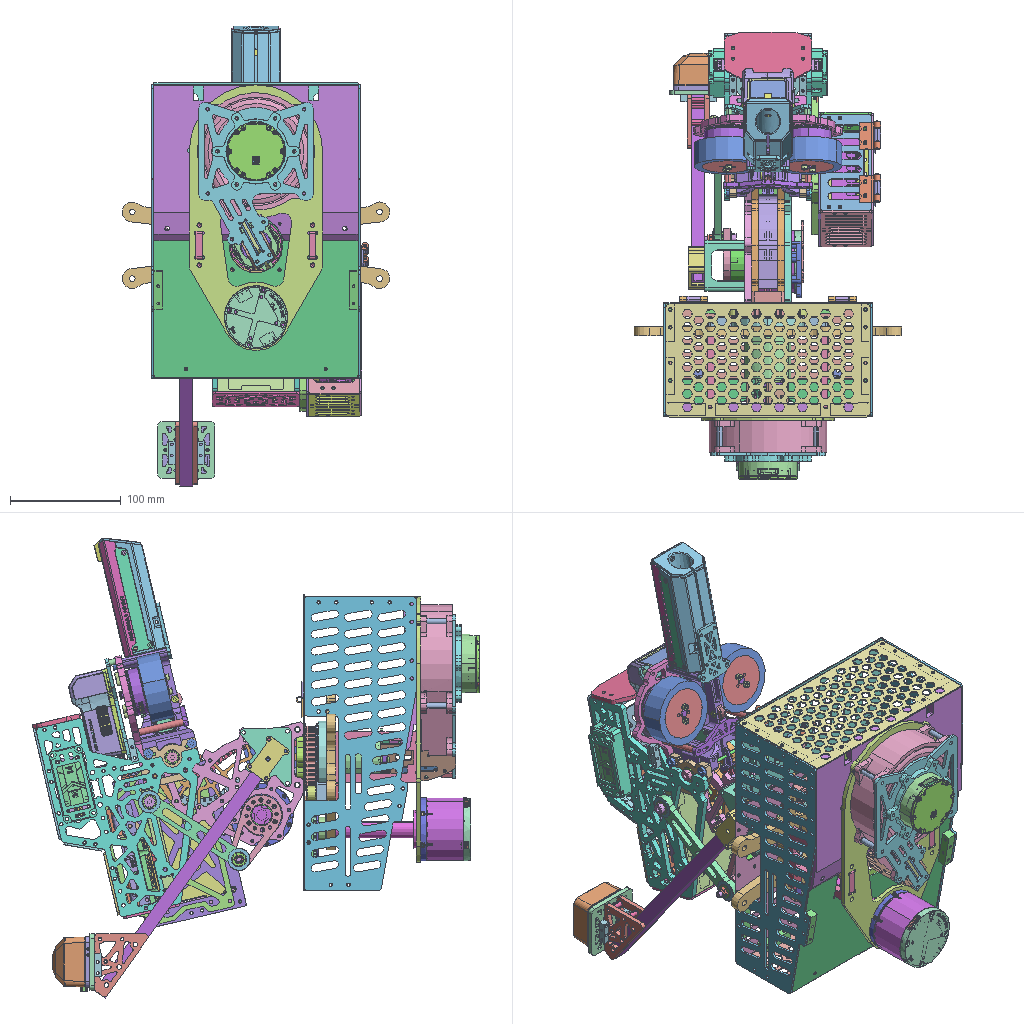Assembly | SolidWorks | 158 different items | 391 placed | box 241 x 403 x 415 mm
Parts list (item | name | quantity | parent item | size | volume | features):
1 | (subassembly) | x1 | in 16 | 129.15 x 61 x 153.15 mm | 192144 mm3 | features CompositeCurve 40
2 | (subassembly) | x1 | in 17 | 67.75 x 214.75 x 243.725 mm | 76567 mm3 | -
3 | (subassembly) | x1 | in 4 | - | 99584 mm3 | -
4 | (subassembly) | x1 | in 15 | - | 170977 mm3 | -
5 | (subassembly) | x1 | in 16 | - | 253666 mm3 | -
6 | (subassembly) | x1 | in 16 | 22 x 68.45 x 50.65 mm | 15273 mm3 | features CompositeCurve 1
7 | (subassembly) | x1 | in 1 | 82.987 x 87 x 9.9 mm | 11718 mm3 | features ReferencePattern 27, LocalCirPattern 1
8 | (subassembly) | x2 | in 15 | 60 x 60 x 46.2 mm | 74410 mm3 | -
9 | (subassembly) | x1 | in 15 | 60 x 48 x 108.75 mm | 39263 mm3 | features CompositeCurve 2
10 | (subassembly) | x1 | in 15 | 178.016 x 263.013 x 465.513 mm | 233417 mm3 | -
11 | (subassembly) | x1 | in 2 | 331.13 x 100 x 331.13 mm | 4244509 mm3 | -
12 | (subassembly) | x1 | in 15 | 100 x 100 x 128.825 mm | 681485 mm3 | -
13 | (subassembly) | x1 | in 16 | 65 x 64.3 x 65 mm | 21867 mm3 | -
14 | (subassembly) | x1 | in 16 | - | 185614 mm3 | -
15 | (subassembly) | x1 | - | - | - | features 3DProfileFeature 1, CenterOfMass 1, CoordSys 1
16 | (subassembly) | x1 | - | - | - | features RefAxis 1
17 | (subassembly) | x1 | - | - | 313010 mm3 | -
18 | - | x1 | in 3 | - | 32010 mm3 | features BaseBody 27
19 | - | x2 | in 6 | 2 x 67.95 x 43.25 mm | 3148 mm3 | features Fillet 2, Extrusion 1
20 | - | x2 | in 6 | 1.5 x 34.486 x 16.15 mm | 467.212 mm3 | features Extrusion 1, Fillet 1
21 | - | x1 | in 6 | 3 x 38.5 x 16.4 mm | 858.003 mm3 | features Fillet 2, Extrusion 1, ICE 1
22 | - | x2 | in 6 | 1.5 x 59.45 x 43.25 mm | 1169 mm3 | features Extrusion 1, Fillet 1
23 | - | x1 | in 6 | 3 x 68.45 x 49.25 mm | 1803 mm3 | features Fillet 2, Extrusion 1, ICE 1
24 | - | x1 | in 7 | 81.787 x 85.8 x 7 mm | 10881 mm3 | features ICE 6, HoleWzd 2, Extrusion 1
25 | - | x1 | in 1 | 103 x 3 x 147.909 mm | 16759 mm3 | features Fillet 3, Extrusion 1, HoleWzd 1, ICE 1
26 | - | x2 | in 8 | 60 x 21 x 60 mm | 35557 mm3 | features ICE 2, Extrusion 1
27 | - | x1 | in 15 | 81 x 4 x 18.75 mm | 2669 mm3 | features Fillet 2, Extrusion 1, ICE 1
28 | - | x4 | in 8 | 5.6 x 13 x 5.6 mm | 135.451 mm3 | features Chamfer 1, Extrusion 1, Fillet 1, ICE 1, StudWizard 1
29 | - | x2 | in 15 | 66 x 14 x 30.5 mm | 6792 mm3 | features ICE 14, Fillet 6, Chamfer 1, Extrusion 1
30 | - | x2 | in 16 | 46 x 84.45 x 6 mm | 10492 mm3 | features Fillet 2, HoleWzd 2, ICE 2, Extrusion 1
31 | - | x2 | in 14, 16 | 28.5 x 4 x 28.5 mm | 1085 mm3 | features Extrusion 1, Fillet 1, ICE 1
32 | - | x10 | in 15 | 13.6 x 4 x 13.6 mm | 365.028 mm3 | features Extrusion 1, ICE 1
33 | - | x1 | in 15 | 38 x 3 x 51.4 mm | 2836 mm3 | features Fillet 2, Extrusion 1, ICE 1
34 | - | x45 | in 17 | 5 x 2 x 5 mm | 32.926 mm3 | features Extrusion 1, Fillet 1
35 | - | x31 | in 1, 6, 7 | 5 x 2.5 x 5 mm | 39.243 mm3 | features ICE 2, Extrusion 1, Fillet 1
36 | - | x1 | in 17 | 9 x 50.866 x 41.619 mm | 7798 mm3 | features Extrusion 1, Fillet 1, ICE 1
37 | - | x1 | in 17 | 44 x 14 x 44 mm | 3465 mm3 | features ICE 5, Extrusion 1, Fillet 1
38 | - | x1 | in 15 | 79 x 44 x 4 mm | 12779 mm3 | features Extrusion 1, Fillet 1
39 | - | x1 | in 15 | 79 x 2 x 34.5 mm | 3709 mm3 | features Fillet 2, Extrusion 1, ICE 1
40 | - | x1 | in 17 | 2 x 52.935 x 33.87 mm | 1610 mm3 | features Extrusion 1, Fillet 1
41 | - | x1 | in 15 | 79 x 2 x 102.5 mm | 10788 mm3 | features Fillet 2, Extrusion 1, ICE 1
42 | - | x2 | in 17 | 4 x 2.5 x 4 mm | 23.497 mm3 | features Chamfer 1, Extrusion 1
43 | - | x1 | - | 8 x 2 x 8 mm | 43.212 mm3 | features Chamfer 1, Extrusion 1
44 | - | x24 | in 2, 4, 15 | 21 x 6 x 6 mm | 638.19 mm3 | features HoleWzd 2, Extrusion 1
45 | - | x6 | in 4, 15 | 30 x 6 x 6 mm | 918.019 mm3 | features HoleWzd 4, Extrusion 1
46 | - | x12 | in 5 | 34 x 8 x 8 mm | 2019 mm3 | features HoleWzd 2, Extrusion 1
47 | - | x3 | in 2 | 5 x 12 x 5 mm | 176.715 mm3 | features Extrusion 1, HoleWzd 1
48 | - | x4 | in 1 | 5 x 18 x 5 mm | 265.072 mm3 | features Extrusion 1, HoleWzd 1
49 | - | x14 | in 6, 15 | 5 x 6 x 5 mm | 88.357 mm3 | features Extrusion 1, HoleWzd 1
50 | - | x2 | in 15 | 6 x 41.2 x 6 mm | 962.663 mm3 | features Extrusion 1, HoleWzd 1
51 | - | x2 | in 14, 17 | 57 x 46 x 57 mm | 102676 mm3 | features BaseBody 10
52 | - | x1 | in 1 | 2 x 22 x 2 mm | 68.88 mm3 | features Chamfer 1, Extrusion 1
53 | - | x2 | in 9 | 60 x 3 x 3 mm | 423.91 mm3 | features Chamfer 1, Extrusion 1
54 | - | x1 | - | 9.083 x 5 x 8 mm | 167.216 mm3 | features Extrusion 1, Fillet 1, ICE 1
55 | - | x7 | in 4, 15 | 19 x 6 x 26 mm | 742.94 mm3 | features ICE 3, Extrusion 1
56 | - | x7 | in 4, 15 | 19 x 6 x 25 mm | 724.19 mm3 | features ICE 2, Extrusion 1
57 | - | x2 | - | 10 x 11.684 x 24.374 mm | 433.075 mm3 | features ICE 2, Extrusion 1, Fillet 1
58 | - | x1 | in 9 | 60 x 48 x 108.75 mm | 35872 mm3 | features ICE 19, Fillet 6, HoleWzd 4, MirrorPattern 4, Chamfer 3, 3DProfileFeature 1, Extrusion 1
59 | - | x2 | in 8 | 42 x 44.967 x 43.4 mm | 38568 mm3 | features BaseBody 24, RefSurface 18
60 | - | x1 | in 1 | 36 x 53 x 53.058 mm | 61188 mm3 | features BaseBody 19
61 | - | x1 | in 1 | 69.8 x 20.5 x 78 mm | 11428 mm3 | features Fillet 2, HoleWzd 2, ICE 2, Extrusion 1
62 | - | x1 | in 16 | 42 x 53 x 63.2 mm | 45858 mm3 | features BaseBody 1
63 | - | x1 | in 15 | 6 x 103 x 144 mm | 23755 mm3 | features Fillet 3, ICE 2, Extrusion 1, HoleWzd 1
64 | - | x1 | in 4 | 88.5 x 2 x 46 mm | 5464 mm3 | features Extrusion 1, Fillet 1, ICE 1
65 | - | x1 | in 5 | 92.5 x 1 x 188 mm | 13106 mm3 | features ICE 2, Extrusion 1, Fillet 1
66 | - | x1 | in 4 | 136 x 2 x 46 mm | 7575 mm3 | features Extrusion 1, Fillet 1, ICE 1
67 | - | x1 | in 4 | 88.5 x 2 x 46 mm | 5379 mm3 | features Extrusion 1, Fillet 1, ICE 1
68 | - | x1 | in 4 | 134 x 2 x 91.5 mm | 16934 mm3 | features Fillet 4, ICE 2, Extrusion 1
69 | - | x1 | in 4 | 136 x 2 x 46 mm | 8461 mm3 | features Fillet 2, Extrusion 1, ICE 1
70 | - | x1 | in 4 | 136 x 2 x 92.5 mm | 14381 mm3 | features Fillet 2, Extrusion 1, ICE 1
71 | - | x1 | - | 116 x 20 x 6 mm | 7064 mm3 | features Extrusion 1, Fillet 1
72 | - | x1 | - | 73 x 36 x 6 mm | 6499 mm3 | features Extrusion 1, Fillet 1, ICE 1
73 | - | x1 | - | 36 x 36 x 22.4 mm | 11568 mm3 | features ICE 2, Chamfer 1, Extrusion 1, HoleWzd 1
74 | - | x2 | in 17 | 20 x 18.4 x 13 mm | 1567 mm3 | features ICE 5, Chamfer 1, Extrusion 1, HoleWzd 1
75 | - | x1 | in 13 | 65 x 7.8 x 65 mm | 10339 mm3 | features Extrusion 1, HoleWzd 1, ICE 1
76 | - | x2 | in 5 | 2 x 101 x 264.6 mm | 30475 mm3 | features ICE 9, Fillet 3, Extrusion 1
77 | - | x2 | in 15 | 53.7 x 11.5 x 26.125 mm | 11767 mm3 | features BaseBody 18
78 | - | x1 | in 11 | 45.5 x 33.5 x 49.567 mm | 18394 mm3 | features BaseBody 3, ICE 1
79 | - | x1 | in 15 | - | 22684 mm3 | features BaseBody 8
80 | - | x1 | in 12 | 43.4 x 42.4 x 109.827 mm | 92437 mm3 | features BaseBody 32
81 | - | x1 | in 15 | - | 15304 mm3 | features BaseBody 37
82 | - | x1 | in 10 | - | - | features RefSurface 185, BaseBody 6
83 | - | x1 | in 3 | 26.5 x 9 x 31.5 mm | 4092 mm3 | features ICE 2, Extrusion 1
84 | - | x2 | in 9 | 13 x 6 x 13 mm | 573.868 mm3 | features ICE 2, Blend 1, Chamfer 1, MirrorPattern 1
85 | - | x1 | in 14 | 239.599 x 4 x 120 mm | 43541 mm3 | features Fillet 3, Extrusion 1
86 | - | x1 | in 13 | 44 x 63.961 x 44 mm | 8169 mm3 | features ICE 3, Chamfer 1, Extrusion 1, Fillet 1, HoleWzd 1
87 | - | x1 | in 5 | 1 x 101.95 x 184 mm | 12597 mm3 | features Fillet 2, ICE 2, APattern 1, Extrusion 1
88 | - | x1 | in 17 | 60.296 x 27.5 x 60.296 mm | 17224 mm3 | features ICE 4, Chamfer 2, CirPattern 1, HoleWzd 1, Revolution 1
89 | - | x1 | in 14 | 56.006 x 9 x 56.006 mm | 12826 mm3 | features ICE 6, Chamfer 1, CirPattern 1, Fillet 1, Revolution 1
90 | - | x1 | in 14 | 60 x 60 x 2 mm | 2571 mm3 | features ICE 3, Extrusion 1, Fillet 1
91 | - | x1 | in 14 | 60 x 60 x 2 mm | 3559 mm3 | features ICE 2, Extrusion 1
92 | - | x1 | in 14 | 35 x 35 x 95.91 mm | 18807 mm3 | features ICE 5, Extrusion 1
93 | - | x1 | in 14 | 22 x 22 x 8.66 mm | 548.531 mm3 | features Chamfer 1, Extrusion 1
94 | - | x2 | in 16 | 30 x 20 x 17 mm | 4794 mm3 | features ICE 5, Fillet 3, Extrusion 1
95 | - | x2 | in 16 | 18 x 6 x 10 mm | 956.762 mm3 | features Extrusion 1, Fillet 1, HoleWzd 1
96 | - | x1 | in 11 | 331.13 x 100 x 331.13 mm | 4226115 mm3 | features Blend 1
97 | - | x1 | in 12 | 100 x 100 x 100 mm | 523599 mm3 | features Revolution 1
98 | - | x1 | in 5 | 1 x 66.5 x 184 mm | 8811 mm3 | features Fillet 2, ICE 2, APattern 1, Extrusion 1
99 | - | x1 | in 12 | 50 x 50 x 50 mm | 65450 mm3 | features Revolution 1
100 | - | x1 | in 10 | 115.47 x 100 x 115.47 mm | 349066 mm3 | features Revolution 1
101 | - | x1 | in 10 | 140 x 140 x 70 mm | 718378 mm3 | features Revolution 1
102 | - | x1 | in 10 | 263.013 x 100 x 465.513 mm | 119004 mm3 | features 3DProfileFeature 5, CirPattern 2, FillRefSurface 2, Thicken 2, RefAxis 1
103 | - | x1 | in 17 | 6 x 130 x 95.37 mm | 22156 mm3 | features ICE 2, Extrusion 1, Fillet 1
104 | - | x1 | in 17 | 6 x 130 x 111.291 mm | 30110 mm3 | features ICE 4, Fillet 3, Extrusion 1
105 | - | x1 | in 16 | 241 x 142.05 x 8 mm | 87619 mm3 | features ICE 6, Fillet 3, Extrusion 1
106 | - | x1 | in 15 | 79 x 2 x 57.5 mm | 5646 mm3 | features Extrusion 1, Fillet 1, ICE 1
107 | - | x1 | in 15 | 79 x 51.5 x 2 mm | 5613 mm3 | features Fillet 5, ICE 3, Extrusion 1
108 | - | x1 | in 13 | 51 x 5 x 51 mm | 3359 mm3 | features ICE 3, Extrusion 1, Fillet 1, RefAxis 1, RevCut 1
109 | - | x1 | in 5 | 148.62 x 27.16 x 184 mm | 24771 mm3 | features ICE 7, Fillet 3, Cut 1, Extrusion 1
110 | - | x1 | in 1 | 122.366 x 28.8 x 124.721 mm | 74874 mm3 | features ICE 18, Fillet 13, Extrusion 1, Shell 1, SweepCut 1
111 | - | x1 | in 6 | 18 x 9.45 x 11 mm | 943.932 mm3 | features ICE 2, Extrusion 1, Fillet 1, HoleWzd 1
112 | - | x10 | in 7 | 3.7 x 9.9 x 3.7 mm | 41.479 mm3 | features ICE 2, Extrusion 1, Fillet 1, StudWizard 1
113 | - | x2 | in 15 | 6.5 x 54 x 35 mm | 7066 mm3 | features HoleWzd 3, Fillet 2, Chamfer 1, Extrusion 1
114 | - | x2 | in 15 | 5 x 138 x 183 mm | 44741 mm3 | features Fillet 3, Extrusion 1, ICE 1
115 | - | x1 | in 15 | 133.928 x 6 x 121.75 mm | 39124 mm3 | features Fillet 3, ICE 2, Extrusion 1
116 | - | x1 | in 15 | 69 x 31.5 x 2 mm | 3100 mm3 | features Fillet 2, Extrusion 1, ICE 1
117 | - | x1 | in 15 | 76 x 10 x 107.5 mm | 24777 mm3 | features HoleWzd 5, Fillet 2, Extrusion 1, ICE 1
118 | - | x1 | in 17 | 60.296 x 5 x 60.296 mm | 2721 mm3 | features Chamfer 2, Extrusion 1, ICE 1
119 | - | x1 | in 15 | 91 x 3 x 91.75 mm | 7865 mm3 | features Fillet 2, Extrusion 1, ICE 1
120 | - | x1 | in 5 | 169.72 x 1 x 93.5 mm | 9219 mm3 | features ICE 12, Fillet 3, Extrusion 1
121 | - | x2 | in 17 | 19.532 x 5 x 19.532 mm | 1006 mm3 | features Chamfer 1, Extrusion 1, HoleWzd 1
122 | - | x1 | in 15 | 5 x 10 x 5 mm | 125.664 mm3 | features Extrusion 1
123 | - | x8 | in 15 | 6.8 x 15.1 x 6.8 mm | 217.57 mm3 | features ICE 2, Chamfer 1, Extrusion 1, StudWizard 1
124 | - | x8 | in 15 | 8.8 x 17.1 x 8.8 mm | 397.168 mm3 | features ICE 2, Chamfer 1, Extrusion 1, StudWizard 1
125 | - | x2 | in 15 | 9.8 x 25.8 x 9.8 mm | 830.154 mm3 | features ICE 2, Chamfer 1, Extrusion 1, StudWizard 1
126 | - | x2 | - | 9.8 x 29.8 x 9.8 mm | 943.251 mm3 | features ICE 2, Chamfer 1, Extrusion 1, StudWizard 1
127 | - | x2 | in 9 | 7 x 7.6 x 7 mm | 97.472 mm3 | features Chamfer 2, Extrusion 1, ICE 1, StudWizard 1
128 | - | x2 | in 9 | 8.5 x 11.5 x 8.5 mm | 159.076 mm3 | features Chamfer 2, ICE 2, Extrusion 1, HoleWzd 1
129 | - | x1 | in 2 | 36 x 45.983 x 53.5 mm | 11586 mm3 | features ICE 9, Fillet 6, HoleWzd 4, Chamfer 1, Extrusion 1
130 | - | x1 | in 2 | 12 x 275 x 12 mm | 21786 mm3 | features ICE 3, Extrusion 1
131 | - | x1 | in 5 | 169.72 x 1 x 93.5 mm | 9219 mm3 | features ICE 12, Fillet 3, Extrusion 1
132 | - | x1 | in 2 | 24.2 x 14.5 x 36 mm | 4824 mm3 | features Fillet 2, ICE 2, Extrusion 1
133 | - | x1 | in 2 | 51.5 x 4 x 51 mm | 7707 mm3 | features Fillet 2, Extrusion 1, HoleWzd 1, ICE 1
134 | - | x2 | in 2 | 56.79 x 52.15 x 4 mm | 5232 mm3 | features Fillet 3, Cut 2, ICE 2, Extrusion 1
135 | - | x1 | in 3 | 126 x 9.5 x 78.6 mm | 28044 mm3 | features Fillet 7, ICE 4, Cut 2, MBimport 1, MirrorPattern 1
136 | - | x1 | in 3 | 113.2 x 30 x 73.2 mm | 35438 mm3 | features BaseBody 1, Chamfer 1, ICE 1
137 | - | x3 | - | 20 x 0.5 x 20 mm | 100.531 mm3 | features Extrusion 1
138 | - | x1 | - | 8 x 8 x 0.5 mm | 10.996 mm3 | features Extrusion 1
139 | - | x6 | in 6 | 3 x 10 x 3 mm | 68.413 mm3 | features ICE 2, Extrusion 1, StudWizard 1
140 | - | x2 | in 16 | 13 x 14 x 13 mm | 1049 mm3 | features Fillet 4, ICE 2, Revolution 2, StudWizard 1
141 | - | x1 | in 1 | 59.347 x 20 x 61.172 mm | 14853 mm3 | features ICE 6, Blend 2, Chamfer 2, Fillet 2, BlendCut 1, Revolution 1
142 | - | x2 | in 5 | 14.084 x 8 x 12.339 mm | 464.267 mm3 | features ICE 3, Extrusion 1
143 | - | x2 | in 5 | 25 x 6 x 19 mm | 560.152 mm3 | features ICE 2, Extrusion 1, MirrorPattern 1
144 | - | x2 | in 5 | 25 x 6 x 19 mm | 560.152 mm3 | features ICE 2, Extrusion 1
145 | - | x10 | in 7 | 3.4 x 0.5 x 3.4 mm | 2.933 mm3 | features Extrusion 1, Fillet 1
146 | - | x4 | in 8 | 4.6 x 0.8 x 4.6 mm | 7.538 mm3 | features Extrusion 1, Fillet 1
147 | - | x1 | in 5 | 184 x 140.059 x 11.963 mm | 87772 mm3 | features ICE 17, 3DProfileFeature 8, Fillet 3, Extrusion 1, MirrorPattern 1
148 | - | x2 | in 17 | 6 x 140.191 x 67.073 mm | 12197 mm3 | features Fillet 2, Extrusion 1, ICE 1
149 | - | x2 | in 17 | 2 x 112.104 x 36.273 mm | 1700 mm3 | features Extrusion 1, Fillet 1
150 | - | x1 | in 17 | 17.6 x 86.542 x 33.473 mm | 4076 mm3 | features Extrusion 1, Fillet 1, HoleWzd 1, ICE 1
151 | - | x2 | in 17 | 2 x 138.567 x 40.786 mm | 2138 mm3 | features Extrusion 1, Fillet 1
152 | - | x1 | in 17 | 17.6 x 113.917 x 33.473 mm | 5862 mm3 | features Extrusion 1, Fillet 1, HoleWzd 1, ICE 1
153 | - | x2 | in 9 | 20 x 5.45 x 12 mm | 441.181 mm3 | features ICE 3, Fillet 2, Extrusion 1, Revolution 1
154 | DM-MC-Board02 电机开发Plate | x1 | - | - | - | -
155 | RoboMaster 红点激光器 RL35 | x1 | - | - | - | -
156 | 定位Bracket侧Plate-碳Plate | x1 | - | - | - | -
157 | 定位BracketPlate-碳Plate | x1 | - | - | - | -
158 | 定位模块安装Plate-碳Plate | x1 | - | - | - | -
Mates (type | each side: item.copy, entity, surface, feature), first 447 of 750 lines:
In the top assembly
Concentric | 74.1 face cylinder M5 Tapped Hole 1 | 125.1 face cylinder M5 机械螺纹 螺柱1
Concentric | 51.1 edge | 73.1 face cylinder Boss-Extrude 1
Coincident | 51.1 face plane 输入1 | 73.1 face plane Boss-Extrude 1
Concentric | 73.1 face cylinder Boss-Extrude 2 | 72.1 face cylinder Boss-Extrude 1
Coincident | 73.1 face plane Boss-Extrude 1 | 72.1 face plane Boss-Extrude 1
Concentric | 73.1 face cylinder M3 Tapped Hole 1 | 72.1 face cylinder Boss-Extrude 1
Concentric | 72.1 face cylinder Boss-Extrude 1 | 32.1 face cylinder Boss-Extrude 2
Concentric | 32.1 face cylinder Boss-Extrude 2 | 137.1 face cylinder Boss-Extrude 1
Coincident | 32.1 face plane Boss-Extrude 1 | 137.1 face plane Boss-Extrude 1
Coincident | 72.1 face plane Boss-Extrude 1 | 137.1 face plane Boss-Extrude 1
Concentric | 72.1 face cylinder Boss-Extrude 1 | 32.2 face cylinder Boss-Extrude 2
Coincident | 72.1 face plane Boss-Extrude 1 | 32.2 face plane Boss-Extrude 1
Coincident | 32.2 face plane Boss-Extrude 1 | 138.1 face plane Boss-Extrude 1
Concentric | 32.1 face cylinder Boss-Extrude 1 | 126.1 face cylinder Boss-Extrude 2
Coincident | 32.1 face plane Boss-Extrude 1 | 126.1 face plane Boss-Extrude 1
Concentric | 138.1 face cylinder Boss-Extrude 1 | 126.1 face cylinder Boss-Extrude 2
Concentric | 71.1 face cylinder Boss-Extrude 1 | 32.3 face cylinder Boss-Extrude 2
Coincident | 71.1 face plane Boss-Extrude 1 | 32.3 face plane Boss-Extrude 1
Concentric | 126.1 face cylinder Boss-Extrude 2 | 32.3 face cylinder Boss-Extrude 1
Coincident | 138.1 face plane Boss-Extrude 1 | 32.3 face plane Boss-Extrude 1
Concentric | 71.1 face cylinder Boss-Extrude 1 | 32.4 face cylinder Boss-Extrude 2
Coincident | 71.1 face plane Boss-Extrude 1 | 137.2 face plane Boss-Extrude 1
Concentric | 32.4 face cylinder Boss-Extrude 2 | 137.2 face cylinder Boss-Extrude 1
Coincident | 32.4 face plane Boss-Extrude 1 | 137.2 face plane Boss-Extrude 1
Concentric | 126.1 face cylinder M5 机械螺纹 螺柱1 | 54.1 face cylinder Boss-Extrude 1
Coincident | 32.4 face plane Boss-Extrude 1 | 54.1 face plane Boss-Extrude 1
Coincident | 71.1 face plane Boss-Extrude 1 | 32.5 face plane Boss-Extrude 1
Concentric | 71.1 face cylinder Boss-Extrude 1 | 32.5 face cylinder Boss-Extrude 2
Concentric | 137.3 face cylinder Boss-Extrude 1 | 32.6 face cylinder Boss-Extrude 2
Coincident | 137.3 face plane Boss-Extrude 1 | 32.6 face plane Boss-Extrude 1
Concentric | 71.1 face cylinder Boss-Extrude 1 | 32.6 face cylinder Boss-Extrude 2
Coincident | 71.1 face plane Boss-Extrude 1 | 137.3 face plane Boss-Extrude 1
Concentric | 32.6 face cylinder Boss-Extrude 1 | 126.2 face cylinder Boss-Extrude 2
Coincident | 32.6 face plane Boss-Extrude 1 | 126.2 face plane Boss-Extrude 1
Concentric | 117.1 face cylinder M5 Tapped Hole 1 | 126.2 face cylinder Boss-Extrude 2
Coincident | 114.1 face plane Boss-Extrude 1 | 43.1 face plane Boss-Extrude 1
Concentric | 126.2 face cylinder Boss-Extrude 2 | 43.1 face cylinder Boss-Extrude 1
Concentric | 74.2 face cylinder Boss-Extrude 5 | 125.2 face cylinder Boss-Extrude 1
Concentric | 151.1 face cylinder Boss-Extrude 1 | 57.1 face cylinder Boss-Extrude 1
DistanceDim | 151.1 face plane Boss-Extrude 1 | 57.1 face plane Cut-Extrude 1
Concentric | 149.1 face cylinder Boss-Extrude 1 | 57.2 face cylinder Boss-Extrude 1
Coincident | 57.1 face plane Boss-Extrude 1 | 57.2 face plane Boss-Extrude 1
Coincident | 53.1 select_type:25 | 57.1 select_type:24
Coincident | 53.2 select_type:25 | 57.2 select_type:24
Concentric | 88.1 face cylinder Cut-Extrude 2 | assembly face | 2 times
Coincident | 88.1 face plane Revolve 1 | assembly face
Concentric | 88.1 face cylinder Cut-Extrude 2 | 86.1 face cylinder M4 Tapped Hole 1 | 2 times
Coincident | 88.1 face plane Revolve 1 | 108.1 face plane Boss-Extrude 1
In subassembly 17
Concentric | 88.2 face cylinder Revolve 1 | 17.1 select_type:11
Coincident | 88.2 face plane Revolve 1 | 17.1 select_type:11
Parallel | 88.2 face plane Boss-Extrude 1 | 17.1 plane
Coincident | 88.2 face plane Revolve 1 | 17.1 plane
Coincident | 88.2 face plane Boss-Extrude 1 | 104.1 face plane Boss-Extrude 1
Concentric | 88.2 face cylinder M5 Tapped Hole 1 | 104.1 face cylinder Boss-Extrude 1 | 2 times
Coincident | 88.2 face plane Boss-Extrude 1 | 103.1 face plane Boss-Extrude 1
Concentric | 88.2 face cylinder M5 Tapped Hole 1 | 103.1 face cylinder Boss-Extrude 1 | 2 times
Coincident | 104.1 face plane Boss-Extrude 1 | 148.1 face plane Boss-Extrude 1
Concentric | 148.1 face cylinder Boss-Extrude 1 | 104.1 face cylinder Cut-Extrude 1
Concentric | 104.1 face cylinder Cut-Extrude 1 | 148.1 face cylinder Boss-Extrude 1
Concentric | 103.1 face cylinder Cut-Extrude 1 | 148.2 face cylinder Boss-Extrude 1 | 2 times
Coincident | 103.1 face plane Boss-Extrude 1 | 148.2 face plane Boss-Extrude 1
Coincident | 148.1 face plane Boss-Extrude 1 | 150.1 face plane Boss-Extrude 2
Concentric | 148.1 face cylinder Boss-Extrude 1 | 150.1 face cylinder M3 Tapped Hole 1 | 2 times
Coincident | 148.1 face plane Boss-Extrude 1 | 152.1 face plane Boss-Extrude 2
Concentric | 148.1 face cylinder Boss-Extrude 1 | 152.1 face cylinder M3 Tapped Hole 1 | 2 times
Coincident | 150.1 face plane Boss-Extrude 1 | 149.2 face plane Boss-Extrude 1
Concentric | 150.1 face cylinder Boss-Extrude 1 | 149.2 face cylinder Boss-Extrude 1 | 2 times
Coincident | 150.1 face plane Boss-Extrude 1 | 149.3 face plane Boss-Extrude 1
Concentric | 150.1 face cylinder Boss-Extrude 1 | 149.3 face cylinder Boss-Extrude 1 | 2 times
Coincident | 152.1 face plane Boss-Extrude 1 | 151.2 face plane Boss-Extrude 1
Concentric | 152.1 face cylinder Boss-Extrude 1 | 151.2 face cylinder Boss-Extrude 1 | 2 times
Coincident | 152.1 face plane Boss-Extrude 1 | 151.3 face plane Boss-Extrude 1
Concentric | 152.1 face cylinder Boss-Extrude 1 | 151.3 face cylinder Boss-Extrude 1 | 2 times
Concentric | 88.2 face cylinder Revolve 1 | 37.1 face cylinder Boss-Extrude 1
Concentric | 88.2 face cylinder Cut-Extrude 2 | 37.1 face cylinder Boss-Extrude 1
Coincident | 104.1 face plane Boss-Extrude 1 | 51.2 face plane 输入4
Concentric | 104.1 face cylinder Boss-Extrude 2 | 51.2 face cylinder 输入1
Concentric | 104.1 face cylinder Boss-Extrude 2 | 51.2 face cone 输入4
Concentric | 149.2 face cylinder Boss-Extrude 1 | 34.1 face cylinder Boss-Extrude 1
DistanceDim | 34.1 face plane Boss-Extrude 1 | 149.2 face plane Boss-Extrude 1
Coincident | 34.1 face plane Boss-Extrude 1 | 34.2 face plane Boss-Extrude 1
Concentric | 149.2 face cylinder Boss-Extrude 1 | 34.2 face cylinder Boss-Extrude 1
Concentric | 149.2 face cylinder Boss-Extrude 1 | 34.3 face cylinder Boss-Extrude 1
Concentric | 149.2 face cylinder Boss-Extrude 1 | 34.4 face cylinder Boss-Extrude 1
Concentric | 149.2 face cylinder Boss-Extrude 1 | 34.5 face cylinder Boss-Extrude 1
Concentric | 149.2 face cylinder Boss-Extrude 1 | 34.6 face cylinder Boss-Extrude 1
Concentric | 149.2 face cylinder Boss-Extrude 1 | 34.7 face cylinder Boss-Extrude 1
Concentric | 149.2 face cylinder Boss-Extrude 1 | 34.8 face cylinder Boss-Extrude 1
Concentric | 149.2 face cylinder Boss-Extrude 1 | 34.9 face cylinder Boss-Extrude 1
Concentric | 149.2 face cylinder Boss-Extrude 1 | 34.10 face cylinder Boss-Extrude 1
Concentric | 149.2 face cylinder Boss-Extrude 1 | 34.11 face cylinder Boss-Extrude 1
Concentric | 149.2 face cylinder Boss-Extrude 1 | 34.12 face cylinder Boss-Extrude 1
Concentric | 149.2 face cylinder Boss-Extrude 1 | 34.13 face cylinder Boss-Extrude 1
Concentric | 149.2 face cylinder Boss-Extrude 1 | 34.14 face cylinder Boss-Extrude 1
Concentric | 149.2 face cylinder Boss-Extrude 1 | 34.15 face cylinder Boss-Extrude 1
Concentric | 149.2 face cylinder Boss-Extrude 1 | 34.16 face cylinder Boss-Extrude 1
Concentric | 149.2 face cylinder Boss-Extrude 1 | 34.17 face cylinder Boss-Extrude 1
Concentric | 149.2 face cylinder Boss-Extrude 1 | 34.18 face cylinder Boss-Extrude 1
Concentric | 149.2 face cylinder Boss-Extrude 1 | 34.19 face cylinder Boss-Extrude 1
Concentric | 151.2 face cylinder Boss-Extrude 1 | 34.20 face cylinder Boss-Extrude 1
Concentric | 151.2 face cylinder Boss-Extrude 1 | 34.21 face cylinder Boss-Extrude 1
Concentric | 151.2 face cylinder Boss-Extrude 1 | 34.22 face cylinder Boss-Extrude 1
Concentric | 151.2 face cylinder Boss-Extrude 1 | 34.23 face cylinder Boss-Extrude 1
Concentric | 151.2 face cylinder Boss-Extrude 1 | 34.24 face cylinder Boss-Extrude 1
Concentric | 151.2 face cylinder Boss-Extrude 1 | 34.25 face cylinder Boss-Extrude 1
Concentric | 151.2 face cylinder Boss-Extrude 1 | 34.26 face cylinder Boss-Extrude 1
Concentric | 151.2 face cylinder Boss-Extrude 1 | 34.27 face cylinder Boss-Extrude 1
Concentric | 151.2 face cylinder Boss-Extrude 1 | 34.28 face cylinder Boss-Extrude 1
Concentric | 151.2 face cylinder Boss-Extrude 1 | 34.29 face cylinder Boss-Extrude 1
Concentric | 151.2 face cylinder Boss-Extrude 1 | 34.30 face cylinder Boss-Extrude 1
Concentric | 151.2 face cylinder Boss-Extrude 1 | 34.31 face cylinder Boss-Extrude 1
Concentric | 151.2 face cylinder Boss-Extrude 1 | 34.32 face cylinder Boss-Extrude 1
Concentric | 151.2 face cylinder Boss-Extrude 1 | 34.33 face cylinder Boss-Extrude 1
Concentric | 151.2 face cylinder Boss-Extrude 1 | 34.34 face cylinder Boss-Extrude 1
Concentric | 151.2 face cylinder Boss-Extrude 1 | 34.35 face cylinder Boss-Extrude 1
Concentric | 151.2 face cylinder Boss-Extrude 1 | 34.36 face cylinder Boss-Extrude 1
Concentric | 151.2 face cylinder Boss-Extrude 1 | 34.37 face cylinder Boss-Extrude 1
Concentric | 151.2 face cylinder Boss-Extrude 1 | 34.38 face cylinder Boss-Extrude 1
Concentric | 151.2 face cylinder Boss-Extrude 1 | 34.39 face cylinder Boss-Extrude 1
Concentric | 151.2 face cylinder Boss-Extrude 1 | 34.40 face cylinder Boss-Extrude 1
Concentric | 151.2 face cylinder Boss-Extrude 1 | 34.41 face cylinder Boss-Extrude 1
Concentric | 151.2 face cylinder Boss-Extrude 1 | 34.42 face cylinder Boss-Extrude 1
Concentric | 151.2 face cylinder Boss-Extrude 1 | 34.43 face cylinder Boss-Extrude 1
Concentric | 151.2 face cylinder Boss-Extrude 1 | 34.44 face cylinder Boss-Extrude 1
Concentric | 151.2 face cylinder Boss-Extrude 1 | 34.45 face cylinder Boss-Extrude 1
Coincident | 34.2 face plane Boss-Extrude 1 | 34.3 face plane Boss-Extrude 1
Coincident | 34.3 face plane Boss-Extrude 1 | 34.4 face plane Boss-Extrude 1
Coincident | 34.4 face plane Boss-Extrude 1 | 34.5 face plane Boss-Extrude 1
Coincident | 34.5 face plane Boss-Extrude 1 | 34.6 face plane Boss-Extrude 1
Coincident | 34.6 face plane Boss-Extrude 1 | 34.7 face plane Boss-Extrude 1
Coincident | 34.7 face plane Boss-Extrude 1 | 34.8 face plane Boss-Extrude 1
Coincident | 34.8 face plane Boss-Extrude 1 | 34.9 face plane Boss-Extrude 1
Coincident | 34.9 face plane Boss-Extrude 1 | 34.10 face plane Boss-Extrude 1
Coincident | 34.10 face plane Boss-Extrude 1 | 34.11 face plane Boss-Extrude 1
Coincident | 34.11 face plane Boss-Extrude 1 | 34.12 face plane Boss-Extrude 1
Coincident | 34.12 face plane Boss-Extrude 1 | 34.13 face plane Boss-Extrude 1
Coincident | 34.13 face plane Boss-Extrude 1 | 34.14 face plane Boss-Extrude 1
Coincident | 34.14 face plane Boss-Extrude 1 | 34.15 face plane Boss-Extrude 1
Coincident | 34.15 face plane Boss-Extrude 1 | 34.16 face plane Boss-Extrude 1
Coincident | 34.16 face plane Boss-Extrude 1 | 34.17 face plane Boss-Extrude 1
Coincident | 34.17 face plane Boss-Extrude 1 | 34.18 face plane Boss-Extrude 1
Coincident | 34.18 face plane Boss-Extrude 1 | 34.19 face plane Boss-Extrude 1
Coincident | 34.1 face plane Boss-Extrude 1 | 34.20 face plane Boss-Extrude 1
Coincident | 34.20 face plane Boss-Extrude 1 | 34.21 face plane Boss-Extrude 1
Coincident | 34.21 face plane Boss-Extrude 1 | 34.22 face plane Boss-Extrude 1
Coincident | 34.22 face plane Boss-Extrude 1 | 34.23 face plane Boss-Extrude 1
Coincident | 34.23 face plane Boss-Extrude 1 | 34.24 face plane Boss-Extrude 1
Coincident | 34.24 face plane Boss-Extrude 1 | 34.25 face plane Boss-Extrude 1
Coincident | 34.25 face plane Boss-Extrude 1 | 34.26 face plane Boss-Extrude 1
Coincident | 34.26 face plane Boss-Extrude 1 | 34.27 face plane Boss-Extrude 1
Coincident | 34.27 face plane Boss-Extrude 1 | 34.28 face plane Boss-Extrude 1
Coincident | 34.29 face plane Boss-Extrude 1 | 34.30 face plane Boss-Extrude 1
Coincident | 34.30 face plane Boss-Extrude 1 | 34.31 face plane Boss-Extrude 1
Coincident | 34.31 face plane Boss-Extrude 1 | 34.32 face plane Boss-Extrude 1
Coincident | 34.32 face plane Boss-Extrude 1 | 34.33 face plane Boss-Extrude 1
Coincident | 34.33 face plane Boss-Extrude 1 | 34.34 face plane Boss-Extrude 1
Coincident | 34.34 face plane Boss-Extrude 1 | 34.35 face plane Boss-Extrude 1
Coincident | 34.35 face plane Boss-Extrude 1 | 34.36 face plane Boss-Extrude 1
Coincident | 34.36 face plane Boss-Extrude 1 | 34.37 face plane Boss-Extrude 1
Coincident | 34.37 face plane Boss-Extrude 1 | 34.38 face plane Boss-Extrude 1
Coincident | 34.38 face plane Boss-Extrude 1 | 34.39 face plane Boss-Extrude 1
Coincident | 34.39 face plane Boss-Extrude 1 | 34.40 face plane Boss-Extrude 1
Coincident | 34.40 face plane Boss-Extrude 1 | 34.41 face plane Boss-Extrude 1
Coincident | 34.41 face plane Boss-Extrude 1 | 34.42 face plane Boss-Extrude 1
Coincident | 34.42 face plane Boss-Extrude 1 | 34.43 face plane Boss-Extrude 1
Coincident | 34.43 face plane Boss-Extrude 1 | 34.44 face plane Boss-Extrude 1
Coincident | 34.44 face plane Boss-Extrude 1 | 34.45 face plane Boss-Extrude 1
Coincident | 34.28 face plane Boss-Extrude 1 | 34.29 face plane Boss-Extrude 1
Coincident | 104.1 face plane Boss-Extrude 1 | 74.3 face plane Boss-Extrude 1
Concentric | 148.1 face cylinder Cut-Extrude 1 | 74.3 face cylinder Boss-Extrude 1
Coincident | 148.1 face plane Cut-Extrude 1 | 74.3 face plane Boss-Extrude 1
Coincident | 103.1 face plane Boss-Extrude 1 | 74.4 face plane Boss-Extrude 1
Concentric | 148.2 face cylinder Cut-Extrude 1 | 74.4 face cylinder Boss-Extrude 1
Coincident | 148.2 face plane Cut-Extrude 1 | 74.4 face plane Boss-Extrude 1
Coincident | 51.2 face plane 输入2 | 40.1 face plane Boss-Extrude 1
Concentric | 51.2 face cylinder 输入2 | 40.1 face cylinder Boss-Extrude 1 | 2 times
Coincident | 151.2 face plane Boss-Extrude 1 | 42.1 face plane Boss-Extrude 1
Concentric | 151.2 face cylinder Boss-Extrude 1 | 42.1 face cylinder Boss-Extrude 1
Coincident | 149.2 face plane Boss-Extrude 1 | 42.2 face plane Boss-Extrude 1
Concentric | 149.2 face cylinder Boss-Extrude 1 | 42.2 face cylinder Boss-Extrude 1
Concentric | 74.3 face cylinder M10×1 细牙螺柱 | 121.1 face cylinder M10x1.0 Tapped Hole 1
Coincident | 104.1 face plane Boss-Extrude 1 | 121.1 face plane Boss-Extrude 1
Concentric | 74.4 face cylinder M10×1 细牙螺柱 | 121.2 face cylinder M10x1.0 Tapped Hole 1
Coincident | 103.1 face plane Boss-Extrude 1 | 121.2 face plane Boss-Extrude 1
Concentric | 88.2 face cylinder Revolve 1 | 118.1 face cylinder Boss-Extrude 1
Coincident | 88.2 face plane Revolve 1 | 118.1 face plane Boss-Extrude 1
Concentric | 104.1 face cylinder Cut-Extrude 1 | 129.1 face cylinder M4 Tapped Hole 1 | 2 times
Coincident | 104.1 face plane Boss-Extrude 1 | 129.1 face plane Boss-Extrude 1
Concentric | 103.1 face cylinder Cut-Extrude 1 | 36.1 face cylinder Boss-Extrude 1 | 2 times
Coincident | 103.1 face plane Boss-Extrude 1 | 36.1 face plane Boss-Extrude 2
In subassembly 2
Coincident | 78.1 face plane 输入3 | 133.1 face plane Boss-Extrude 1
Concentric | 78.1 face cylinder 输入3 | 133.1 face cylinder Boss-Extrude 1 | 2 times
Concentric | 44.1 face cylinder M3 Tapped Hole 2 | 133.1 face cylinder Boss-Extrude 1 | 2 times
Coincident | 44.1 face plane Boss-Extrude 1 | 133.1 face plane Boss-Extrude 1
Concentric | 44.2 face cylinder M3 Tapped Hole 2 | 133.1 face cylinder Boss-Extrude 1 | 2 times
Coincident | 44.2 face plane Boss-Extrude 1 | 133.1 face plane Boss-Extrude 1
Coincident | 130.1 edge | 133.1 edge
Parallel | 129.2 face plane Boss-Extrude 1 | 133.1 face plane Boss-Extrude 1
Coincident | 130.1 face plane Boss-Extrude 1 | 134.1 face plane Boss-Extrude 1 | 2 times
Coincident | 133.1 face plane Boss-Extrude 1 | 134.1 face plane Boss-Extrude 1
Concentric | 130.1 face cylinder Cut-Extrude 2 | 134.2 face cylinder Cut-Extrude 1 | 2 times
Coincident | 130.1 face plane Boss-Extrude 1 | 134.2 face plane Boss-Extrude 1
Concentric | 134.2 face cylinder Cut-Extrude 2 | 47.1 face cylinder M3 Tapped Hole 1
Concentric | 134.2 face cylinder Cut-Extrude 2 | 47.2 face cylinder M3 Tapped Hole 1
Concentric | 134.2 face cylinder Cut-Extrude 2 | 47.3 face cylinder M3 Tapped Hole 1
Coincident | 134.2 face plane Boss-Extrude 1 | 47.1 face plane Boss-Extrude 1
Coincident | 134.2 face plane Boss-Extrude 1 | 47.2 face plane Boss-Extrude 1
Coincident | 134.2 face plane Boss-Extrude 1 | 47.3 face plane Boss-Extrude 1
Coincident | 134.2 face plane Boss-Extrude 1 | 44.1 face plane Boss-Extrude 1
Coincident | 132.1 face plane Boss-Extrude 1 | 130.1 face plane Boss-Extrude 1
Concentric | 132.1 face cylinder Cut-Extrude 1 | 130.1 face cylinder Cut-Extrude 2
Parallel | 132.1 face plane Boss-Extrude 1 | 130.1 face plane Boss-Extrude 1
Coincident | 129.2 face plane Boss-Extrude 1 | 130.1 face plane Boss-Extrude 1
Concentric | 129.2 face cylinder M3 Tapped Hole 1 | 132.1 face cylinder Cut-Extrude 1
In subassembly 11
Coincident | 78.2 face plane 输入3 | 96.1 face plane 放样1
Coincident | 78.2 edge | 96.1 edge | 2 times
In subassembly 15
Parallel | 117.2 face plane Boss-Extrude 1 | 15.1 plane | 2 times
Coincident | 117.2 face plane Boss-Extrude 1 | 114.2 face plane Boss-Extrude 1
Concentric | 114.2 face cylinder Boss-Extrude 1 | 32.4 face cylinder Boss-Extrude 2
Concentric | 32.1 face cylinder Boss-Extrude 1 | 125.3 face cylinder Boss-Extrude 2
Coincident | 32.1 face plane Boss-Extrude 1 | 125.3 face plane Boss-Extrude 1
Concentric | 32.4 face cylinder Boss-Extrude 1 | 125.4 face cylinder Boss-Extrude 2
Coincident | 32.4 face plane Boss-Extrude 1 | 125.4 face plane Boss-Extrude 1
Coincident | 117.2 face plane Boss-Extrude 1 | 79.1 face plane mounting_the_board_type_c_asm(202001072134)-1/3_0-1-solid1
Concentric | 117.2 face cylinder M2.5 Tapped Hole 1 | 79.1 face cylinder mounting_the_board_type_c_asm(202001072134)-1/4_0-4-solid1
Concentric | 117.2 face cylinder M2.5 Tapped Hole 1 | 79.1 face cylinder mounting_the_board_type_c_asm(202001072134)-1/4_0-2-solid1
Coincident | 79.1 face plane mounting_the_board_type_c_asm(202001072134)-1/2_0-1-solid1 | 81.1 face plane RM_ESC_Center_Board2(2)-1/SHELL_DOWN-1-solid1
Concentric | 79.1 face cylinder mounting_the_board_type_c_asm(202001072134)-1/4_0-4-solid1 | 81.1 face cylinder RM_ESC_Center_Board2(2)-1/CENTER_DISTRIBUTION_BOARD-1-solid1
Concentric | 79.1 face cylinder mounting_the_board_type_c_asm(202001072134)-1/4_0-2-solid1 | 81.1 face cylinder RM_ESC_Center_Board2(2)-1/CENTER_DISTRIBUTION_BOARD-1-solid1
Concentric | 59.1 face cylinder RoboMaster M3508 P19直流无刷减速电机.stp-1/1_1.stp-1-solid1 | 115.1 face cylinder Boss-Extrude 1 | 2 times
Coincident | 59.1 face plane RoboMaster M3508 P19直流无刷减速电机.stp-1/1_1.stp-1-solid1 | 115.1 face plane Boss-Extrude 1
Concentric | 59.2 face cylinder RoboMaster M3508 P19直流无刷减速电机.stp-1/1_1.stp-1-solid1 | 115.1 face cylinder Boss-Extrude 1 | 2 times
Coincident | 59.2 face plane RoboMaster M3508 P19直流无刷减速电机.stp-1/1_1.stp-1-solid1 | 115.1 face plane Boss-Extrude 1
Concentric | 82.1 face cylinder 曲Face-输入71 | 119.1 face cylinder Boss-Extrude 1
Concentric | 82.1 face cylinder 曲Face-输入47 | 119.1 face cylinder Boss-Extrude 1
Coincident | 82.1 face plane 曲Face-输入47 | 119.1 face plane Boss-Extrude 1
Coincident | 117.2 face plane Boss-Extrude 1 | 114.3 face plane Boss-Extrude 1
Concentric | 117.2 face cylinder M5 Tapped Hole 1 | 114.3 face cylinder Boss-Extrude 1
Concentric | 119.1 face cylinder Boss-Extrude 1 | 44.1 face cylinder M3 Tapped Hole 2 | 2 times
Coincident | 119.1 face plane Boss-Extrude 1 | 44.1 face plane Boss-Extrude 1
Concentric | 117.2 face cylinder M5 Tapped Hole 1 | 114.2 face cylinder Boss-Extrude 1
Concentric | 32.1 face cylinder Boss-Extrude 2 | 113.1 face cylinder Boss-Extrude 1
Coincident | 32.1 face plane Boss-Extrude 1 | 113.1 face plane Boss-Extrude 1
Concentric | 32.2 face cylinder Boss-Extrude 2 | 113.1 face cylinder Boss-Extrude 1
Concentric | 32.4 face cylinder Boss-Extrude 2 | 113.2 face cylinder Boss-Extrude 1
Coincident | 32.4 face plane Boss-Extrude 1 | 113.2 face plane Boss-Extrude 1
Coincident | 114.3 face plane Boss-Extrude 1 | 113.1 face plane Boss-Extrude 1
Concentric | 32.3 face cylinder Boss-Extrude 2 | 113.2 face cylinder Boss-Extrude 1
Coincident | 32.3 face plane Boss-Extrude 1 | 113.2 face plane Boss-Extrude 1
Concentric | 117.2 face cylinder M4 Tapped Hole 2 | 114.2 face cylinder Boss-Extrude 1
Coincident | 114.3 face plane Boss-Extrude 1 | 44.1 face plane Boss-Extrude 1
Concentric | 114.3 face cylinder Boss-Extrude 1 | 44.1 face cylinder M3 Tapped Hole 1 | 2 times
Concentric | 119.1 face cylinder Boss-Extrude 1 | 44.2 face cylinder M3 Tapped Hole 2 | 2 times
Coincident | 119.1 face plane Boss-Extrude 1 | 44.2 face plane Boss-Extrude 1
Concentric | 117.2 face cylinder M4 Tapped Hole 1 | 114.3 face cylinder Boss-Extrude 1
Concentric | 114.3 face cylinder Boss-Extrude 1 | 113.1 face cylinder M3 Tapped Hole 1
Concentric | 115.1 face cylinder Boss-Extrude 1 | 49.1 face cylinder M3 Tapped Hole 1
Coincident | 115.1 face plane Boss-Extrude 1 | 49.1 face plane Boss-Extrude 1
Concentric | 115.1 face cylinder Boss-Extrude 1 | 49.2 face cylinder M3 Tapped Hole 1
Coincident | 115.1 face plane Boss-Extrude 1 | 49.2 face plane Boss-Extrude 1
Concentric | 44.3 face cylinder M3 Tapped Hole 2 | 41.1 face cylinder Boss-Extrude 1 | 2 times
Coincident | 44.3 face plane Boss-Extrude 1 | 41.1 face plane Boss-Extrude 1
Concentric | 117.2 face cylinder M3 Tapped Hole 1 | 107.1 face cylinder Boss-Extrude 1 | 2 times
Coincident | 117.2 face plane Boss-Extrude 1 | 107.1 face plane Boss-Extrude 1
Concentric | 39.1 face cylinder Boss-Extrude 1 | 44.4 face cylinder M3 Tapped Hole 2 | 2 times
Coincident | 39.1 face plane Boss-Extrude 1 | 44.4 face plane Boss-Extrude 1
Concentric | 114.3 face cylinder Boss-Extrude 1 | 44.5 face cylinder M3 Tapped Hole 1 | 2 times
Coincident | 114.3 face plane Boss-Extrude 1 | 44.5 face plane Boss-Extrude 1
Concentric | 114.2 face cylinder Boss-Extrude 1 | 44.6 face cylinder M3 Tapped Hole 1 | 2 times
Coincident | 114.2 face plane Boss-Extrude 1 | 44.6 face plane Boss-Extrude 1
Concentric | 44.5 face cylinder M3 Tapped Hole 2 | 106.1 face cylinder Boss-Extrude 1 | 2 times
Coincident | 44.5 face plane Boss-Extrude 1 | 106.1 face plane Boss-Extrude 1
Concentric | 41.1 face cylinder Boss-Extrude 1 | 56.1 face cylinder Cut-Extrude 2 | 2 times
Coincident | 41.1 face plane Boss-Extrude 1 | 56.1 face plane Boss-Extrude 1
Concentric | 39.1 face cylinder Boss-Extrude 1 | 55.1 face cylinder Cut-Extrude 2 | 2 times
Coincident | 39.1 face plane Boss-Extrude 1 | 55.1 face plane Boss-Extrude 1
Concentric | 39.1 face cylinder Boss-Extrude 1 | 56.2 face cylinder Cut-Extrude 2 | 2 times
Coincident | 39.1 face plane Boss-Extrude 1 | 56.2 face plane Boss-Extrude 1
Concentric | 106.1 face cylinder Boss-Extrude 1 | 55.2 face cylinder Cut-Extrude 2 | 2 times
Coincident | 106.1 face plane Boss-Extrude 1 | 55.2 face plane Boss-Extrude 1
Concentric | 106.1 face cylinder Boss-Extrude 1 | 56.3 face cylinder Cut-Extrude 2 | 2 times
Coincident | 106.1 face plane Boss-Extrude 1 | 56.3 face plane Boss-Extrude 1
Concentric | 107.1 face cylinder Boss-Extrude 1 | 55.3 face cylinder Cut-Extrude 2 | 2 times
Coincident | 107.1 face plane Boss-Extrude 1 | 55.3 face plane Boss-Extrude 1
Coincident | 114.3 face plane Boss-Extrude 1 | 63.1 face plane Boss-Extrude 1
Concentric | 114.3 face cylinder Boss-Extrude 1 | 63.1 face cylinder Boss-Extrude 1 | 2 times
Concentric | 70.1 face cylinder Boss-Extrude 1 | 63.1 face cylinder Boss-Extrude 1 | 2 times
Coincident | 70.1 face plane Boss-Extrude 1 | 63.1 face plane Boss-Extrude 1
Concentric | 56.4 face cylinder Cut-Extrude 2 | 63.1 face cylinder Boss-Extrude 1 | 2 times
Concentric | 56.5 face cylinder Cut-Extrude 2 | 63.1 face cylinder Boss-Extrude 1 | 2 times
Coincident | 56.4 face plane Boss-Extrude 1 | 63.1 face plane Cut-Extrude 1
Coincident | 56.5 face plane Boss-Extrude 1 | 63.1 face plane Cut-Extrude 1
Coincident | 114.3 face plane Boss-Extrude 1 | 44.7 face plane Boss-Extrude 1
Concentric | 114.3 face cylinder Boss-Extrude 1 | 44.7 face cylinder M3 Tapped Hole 1 | 2 times
Coincident | 114.2 face plane Boss-Extrude 1 | 44.8 face plane Boss-Extrude 1
Concentric | 114.2 face cylinder Boss-Extrude 1 | 44.8 face cylinder M3 Tapped Hole 1 | 2 times
Coincident | 9.1 select_type:25 | 15.1 select_type:11
Parallel | 58.1 face plane 主体 | 15.1 plane | 2 times
Coincident | 58.1 face plane 主体 | 80.1 face plane 输入8
Concentric | 58.1 face cylinder 枪管 | 80.1 face cylinder 输入8
Coincident | 80.1 face plane 输入8 | 33.1 face plane Boss-Extrude 1
Concentric | 58.1 face cylinder Upper部M4 Tapped Hole | 33.1 face cylinder Boss-Extrude 1 | 2 times
Concentric | 113.1 face cylinder Boss-Extrude 1 | 58.1 face cylinder 侧Face M4 Tapped Hole | 2 times
Coincident | 113.1 face plane Boss-Extrude 1 | 58.1 face plane 主体
Coincident | 115.1 face plane Boss-Extrude 1 | 58.1 face plane 主体
Concentric | 115.1 face cylinder Boss-Extrude 1 | 58.1 face cylinder Upper部M4 Tapped Hole | 2 times
Coincident | 114.2 face plane Boss-Extrude 1 | 113.2 face plane Boss-Extrude 1
Concentric | 113.2 face cylinder Boss-Extrude 1 | 58.1 face cylinder 侧Face M4 Tapped Hole
Concentric | 114.3 face cylinder Boss-Extrude 1 | 45.1 face cylinder M3 Tapped Hole 1 | 2 times
Coincident | 114.3 face plane Boss-Extrude 1 | 45.1 face plane Boss-Extrude 1
Concentric | 114.2 face cylinder Boss-Extrude 1 | 45.2 face cylinder M3 Tapped Hole 1 | 2 times
Coincident | 114.2 face plane Boss-Extrude 1 | 45.2 face plane Boss-Extrude 1
Concentric | 38.1 face cylinder Boss-Extrude 1 | 45.1 face cylinder M3 Tapped Hole 2 | 2 times
Coincident | 38.1 face plane Boss-Extrude 1 | 45.1 face plane Boss-Extrude 1
Concentric | 114.3 face cylinder Boss-Extrude 1 | 44.3 face cylinder M3 Tapped Hole 1 | 2 times
Coincident | 114.3 face plane Boss-Extrude 1 | 44.3 face plane Boss-Extrude 1
Coincident | 114.2 face plane Boss-Extrude 1 | 44.9 face plane Boss-Extrude 1
Concentric | 114.2 face cylinder Boss-Extrude 1 | 44.9 face cylinder M3 Tapped Hole 1 | 2 times
Concentric | 114.3 face cylinder Boss-Extrude 1 | 44.4 face cylinder M3 Tapped Hole 1 | 2 times
Coincident | 114.3 face plane Boss-Extrude 1 | 44.4 face plane Boss-Extrude 1
Concentric | 114.2 face cylinder Boss-Extrude 1 | 44.10 face cylinder M3 Tapped Hole 1 | 2 times
Coincident | 114.2 face plane Boss-Extrude 1 | 44.10 face plane Boss-Extrude 1
Coincident | 113.1 face plane Boss-Extrude 1 | 32.2 face plane Boss-Extrude 1
Coincident | 58.1 face plane UpperLower切穿 | 27.1 face plane Boss-Extrude 1
Concentric | 115.1 face cylinder Boss-Extrude 1 | 27.1 face cylinder Boss-Extrude 1 | 2 times
Concentric | 115.1 face cylinder Boss-Extrude 1 | 50.1 face cylinder M3 Tapped Hole 1
Coincident | 115.1 face plane Boss-Extrude 1 | 50.1 face plane Boss-Extrude 1
Concentric | 115.1 face cylinder Boss-Extrude 1 | 50.2 face cylinder M3 Tapped Hole 1
Coincident | 115.1 face plane Boss-Extrude 1 | 50.2 face plane Boss-Extrude 1
Concentric | 113.1 face cylinder Boss-Extrude 1 | 124.1 face cylinder Boss-Extrude 2
Coincident | 113.1 face plane Boss-Extrude 1 | 124.1 face plane Boss-Extrude 1
Concentric | 113.1 face cylinder Boss-Extrude 1 | 124.2 face cylinder Boss-Extrude 2
Coincident | 113.1 face plane Boss-Extrude 1 | 124.2 face plane Boss-Extrude 1
Concentric | 113.2 face cylinder Boss-Extrude 1 | 124.3 face cylinder Boss-Extrude 2
Coincident | 113.2 face plane Boss-Extrude 1 | 124.3 face plane Boss-Extrude 1
Concentric | 113.2 face cylinder Boss-Extrude 1 | 124.4 face cylinder Boss-Extrude 2
Coincident | 113.2 face plane Boss-Extrude 1 | 124.4 face plane Boss-Extrude 1
Concentric | 115.1 face cylinder Boss-Extrude 1 | 124.5 face cylinder Boss-Extrude 2
Coincident | 115.1 face plane Boss-Extrude 1 | 124.5 face plane Boss-Extrude 1
Concentric | 115.1 face cylinder Boss-Extrude 1 | 124.6 face cylinder Boss-Extrude 2
Coincident | 115.1 face plane Boss-Extrude 1 | 124.6 face plane Boss-Extrude 1
Concentric | 115.1 face cylinder Boss-Extrude 1 | 124.7 face cylinder Boss-Extrude 2
Coincident | 115.1 face plane Boss-Extrude 1 | 124.7 face plane Boss-Extrude 1
Concentric | 115.1 face cylinder Boss-Extrude 1 | 124.8 face cylinder Boss-Extrude 2
Coincident | 115.1 face plane Boss-Extrude 1 | 124.8 face plane Boss-Extrude 1
Concentric | 115.1 face cylinder Boss-Extrude 1 | 123.1 face cylinder Boss-Extrude 2
Coincident | 115.1 face plane Boss-Extrude 1 | 123.1 face plane Boss-Extrude 1
Concentric | 115.1 face cylinder Boss-Extrude 1 | 123.2 face cylinder Boss-Extrude 2
Coincident | 115.1 face plane Boss-Extrude 1 | 123.2 face plane Boss-Extrude 1
Concentric | 115.1 face cylinder Boss-Extrude 1 | 123.3 face cylinder Boss-Extrude 2
Coincident | 115.1 face plane Boss-Extrude 1 | 123.3 face plane Boss-Extrude 1
Concentric | 115.1 face cylinder Boss-Extrude 1 | 123.4 face cylinder Boss-Extrude 2
Coincident | 115.1 face plane Boss-Extrude 1 | 123.4 face plane Boss-Extrude 1
Concentric | 115.1 face cylinder Boss-Extrude 1 | 123.5 face cylinder Boss-Extrude 2
Coincident | 115.1 face plane Boss-Extrude 1 | 123.5 face plane Boss-Extrude 1
Concentric | 115.1 face cylinder Boss-Extrude 1 | 123.6 face cylinder Boss-Extrude 2
Coincident | 115.1 face plane Boss-Extrude 1 | 123.6 face plane Boss-Extrude 1
Concentric | 115.1 face cylinder Boss-Extrude 1 | 123.7 face cylinder Boss-Extrude 2
Coincident | 115.1 face plane Boss-Extrude 1 | 123.7 face plane Boss-Extrude 1
Concentric | 115.1 face cylinder Boss-Extrude 1 | 123.8 face cylinder Boss-Extrude 2
Coincident | 115.1 face plane Boss-Extrude 1 | 123.8 face plane Boss-Extrude 1
Coincident | 114.2 face plane Boss-Extrude 1 | 77.1 face plane C620无刷电机调速器(2)-1/7-1-solid1
Concentric | 114.2 face cylinder Boss-Extrude 1 | 77.1 face cylinder C620无刷电机调速器(2)-1/7-1-solid1 | 2 times
Concentric | 114.3 face cylinder Boss-Extrude 1 | 77.2 face cylinder C620无刷电机调速器(2)-1/7-1-solid1 | 2 times
Coincident | 114.3 face plane Boss-Extrude 1 | 77.2 face plane C620无刷电机调速器(2)-1/7-1-solid1
Concentric | 114.3 face cylinder Boss-Extrude 1 | 44.11 face cylinder M3 Tapped Hole 1 | 2 times
Coincident | 114.3 face plane Boss-Extrude 1 | 44.11 face plane Boss-Extrude 1
Concentric | 114.2 face cylinder Boss-Extrude 1 | 44.12 face cylinder M3 Tapped Hole 1 | 2 times
Coincident | 114.2 face plane Boss-Extrude 1 | 44.12 face plane Boss-Extrude 1
Coincident | 44.11 face plane Boss-Extrude 1 | 116.1 face plane Boss-Extrude 1
Concentric | 44.11 face cylinder M3 Tapped Hole 2 | 116.1 face cylinder Boss-Extrude 1 | 2 times
Coincident | 114.3 face plane Boss-Extrude 1 | 29.1 face plane Boss-Extrude 1
Concentric | 114.3 face cylinder Boss-Extrude 1 | 29.1 face cylinder Boss-Extrude 1 | 2 times
Coincident | 114.2 face plane Boss-Extrude 1 | 29.2 face plane Boss-Extrude 1
Concentric | 114.2 face cylinder Boss-Extrude 1 | 29.2 face cylinder Boss-Extrude 1 | 2 times
Concentric | 114.3 face cylinder Boss-Extrude 1 | 44.13 face cylinder M3 Tapped Hole 1 | 2 times
Coincident | 114.3 face plane Boss-Extrude 1 | 44.13 face plane Boss-Extrude 1
Concentric | 114.2 face cylinder Boss-Extrude 1 | 44.14 face cylinder M3 Tapped Hole 1 | 2 times
Coincident | 114.2 face plane Boss-Extrude 1 | 44.14 face plane Boss-Extrude 1
Concentric | 82.1 face cylinder 曲Face-输入47 | 122.1 face cylinder Boss-Extrude 1
Coincident | 82.1 face plane 曲Face-输入48 | 122.1 face plane Boss-Extrude 1
In subassembly 8
Concentric | 59.3 face cylinder RoboMaster M3508 P19直流无刷减速电机.stp-1/1_1.stp-1-solid1 | 26.1 face cylinder Boss-Extrude 1 | 3 times
Coincident | 59.3 face plane RoboMaster M3508 P19直流无刷减速电机.stp-1/1_1.stp-1-solid1 | 26.1 face plane Boss-Extrude 1
Concentric | 26.1 face cylinder Boss-Extrude 1 | 28.1 face cylinder M3 机械螺纹 螺柱1
Concentric | 26.1 face cylinder Boss-Extrude 1 | 28.2 face cylinder M3 机械螺纹 螺柱1
Concentric | 28.1 face cylinder M3 机械螺纹 螺柱1 | 146.1 face cylinder Boss-Extrude 1
Concentric | 28.2 face cylinder M3 机械螺纹 螺柱1 | 146.2 face cylinder Boss-Extrude 1
Coincident | 26.1 face plane Boss-Extrude 1 | 146.2 face plane Boss-Extrude 1
Coincident | 26.1 face plane Boss-Extrude 1 | 146.1 face plane Boss-Extrude 1
Coincident | 28.2 face plane Boss-Extrude 1 | 146.2 face plane Boss-Extrude 1
Coincident | 28.1 face plane Boss-Extrude 1 | 146.1 face plane Boss-Extrude 1
In subassembly 9
Concentric | 58.2 face cylinder 单侧pitch轴线&销轴Hole位 | 53.3 face cylinder Boss-Extrude 1
Concentric | 58.2 face cylinder 单侧pitch轴线&销轴Hole位 | 53.4 face cylinder Boss-Extrude 1
Concentric | 58.2 face cylinder 单发限位安装Hole | 84.1 face cylinder Cut-Extrude 1
Concentric | 58.2 face cylinder 单发限位安装Hole | 84.2 face cylinder Cut-Extrude 1
Coincident | 84.1 edge | 9.2 plane
Coincident | 84.2 edge | 9.2 plane
Concentric | 128.1 face cylinder M3 Tapped Hole 1 | 127.1 face cylinder M3 机械螺纹 螺柱1
Concentric | 128.2 face cylinder M3 Tapped Hole 1 | 127.2 face cylinder M3 机械螺纹 螺柱1
Coincident | 58.2 face plane 主体 | 128.1 face plane Boss-Extrude 1
Coincident | 58.2 face plane 主体 | 127.1 face plane Boss-Extrude 1
Coincident | 58.2 face plane 主体 | 128.2 face plane Boss-Extrude 1
Coincident | 58.2 face plane 主体 | 127.2 face plane Boss-Extrude 1
Coincident | 53.3 face plane Boss-Extrude 1 | 53.4 face plane Boss-Extrude 1
Coincident | 53.3 select_type:25 | 9.2 plane
Coincident | 58.2 select_type:25 | 9.2 select_type:11
Parallel | 58.2 face plane 主体 | 9.2 plane
Concentric | 58.2 face cylinder 单发限位安装Hole | 128.1 face cylinder Boss-Extrude 2
Concentric | 58.2 face cylinder 单发限位安装Hole | 128.2 face cylinder Boss-Extrude 2
Concentric | 58.2 face cylinder 荧光充能M2.5 Tapped Hole | 153.1 face cylinder 螺丝Hole | 2 times
Coincident | 58.2 face plane 单侧荧光充能铝基Plate镂空 | 153.1 face plane 铝基Plate
Concentric | 58.2 face cylinder 荧光充能M2.5 Tapped Hole | 153.2 face cylinder 螺丝Hole | 2 times
Coincident | 58.2 face plane 对侧荧光充能铝基Plate镂空 | 153.2 face plane 铝基Plate
In subassembly 12
Coordinate | 99.1 select_type:25 | 12.1 select_type:11
Coordinate | 99.1 select_type:25 | 97.1 select_type:25
In subassembly 4
Coincident | 135.1 face plane Boss-Extrude 3 | 70.2 face plane Boss-Extrude 1
Concentric | 135.1 face cylinder Boss-Extrude 2 | 70.2 face cylinder Boss-Extrude 1
Concentric | 135.1 face cylinder Mirror 1 | 70.2 face cylinder Boss-Extrude 1
Coincident | 70.2 face plane Boss-Extrude 1 | 44.1 face plane Boss-Extrude 1
Coincident | 70.2 face plane Boss-Extrude 1 | 44.2 face plane Boss-Extrude 1
Concentric | 70.2 face cylinder Boss-Extrude 1 | 44.2 face cylinder M3 Tapped Hole 2 | 2 times
Coincident | 70.2 face plane Boss-Extrude 1 | 44.9 face plane Boss-Extrude 1
Concentric | 70.2 face cylinder Boss-Extrude 1 | 44.9 face cylinder M3 Tapped Hole 2 | 2 times
Concentric | 70.2 face cylinder Boss-Extrude 1 | 44.1 face cylinder M3 Tapped Hole 2 | 2 times
Coincident | 70.2 face plane Boss-Extrude 1 | 44.15 face plane Boss-Extrude 1
Coincident | 70.2 face plane Boss-Extrude 1 | 45.1 face plane Boss-Extrude 1
Concentric | 70.2 face cylinder Boss-Extrude 1 | 45.1 face cylinder M3 Tapped Hole 3
Concentric | 70.2 face cylinder Boss-Extrude 1 | 45.2 face cylinder M3 Tapped Hole 3
Coincident | 70.2 face plane Boss-Extrude 1 | 45.2 face plane Boss-Extrude 1
Concentric | 70.2 face cylinder Boss-Extrude 1 | 45.3 face cylinder M3 Tapped Hole 3
Coincident | 70.2 face plane Boss-Extrude 1 | 45.3 face plane Boss-Extrude 1
Concentric | 70.2 face cylinder Boss-Extrude 1 | 45.4 face cylinder M3 Tapped Hole 3
Coincident | 70.2 face plane Boss-Extrude 1 | 45.4 face plane Boss-Extrude 1
Coincident | 45.2 face plane Boss-Extrude 1 | 66.1 face plane Boss-Extrude 1
Concentric | 45.2 face cylinder M3 Tapped Hole 1 | 66.1 face cylinder Boss-Extrude 1
Concentric | 45.3 face cylinder M3 Tapped Hole 1 | 66.1 face cylinder Boss-Extrude 1
Coincident | 45.1 face plane Boss-Extrude 1 | 67.1 face plane Boss-Extrude 1
Concentric | 45.2 face cylinder M3 Tapped Hole 2 | 67.1 face cylinder Boss-Extrude 1